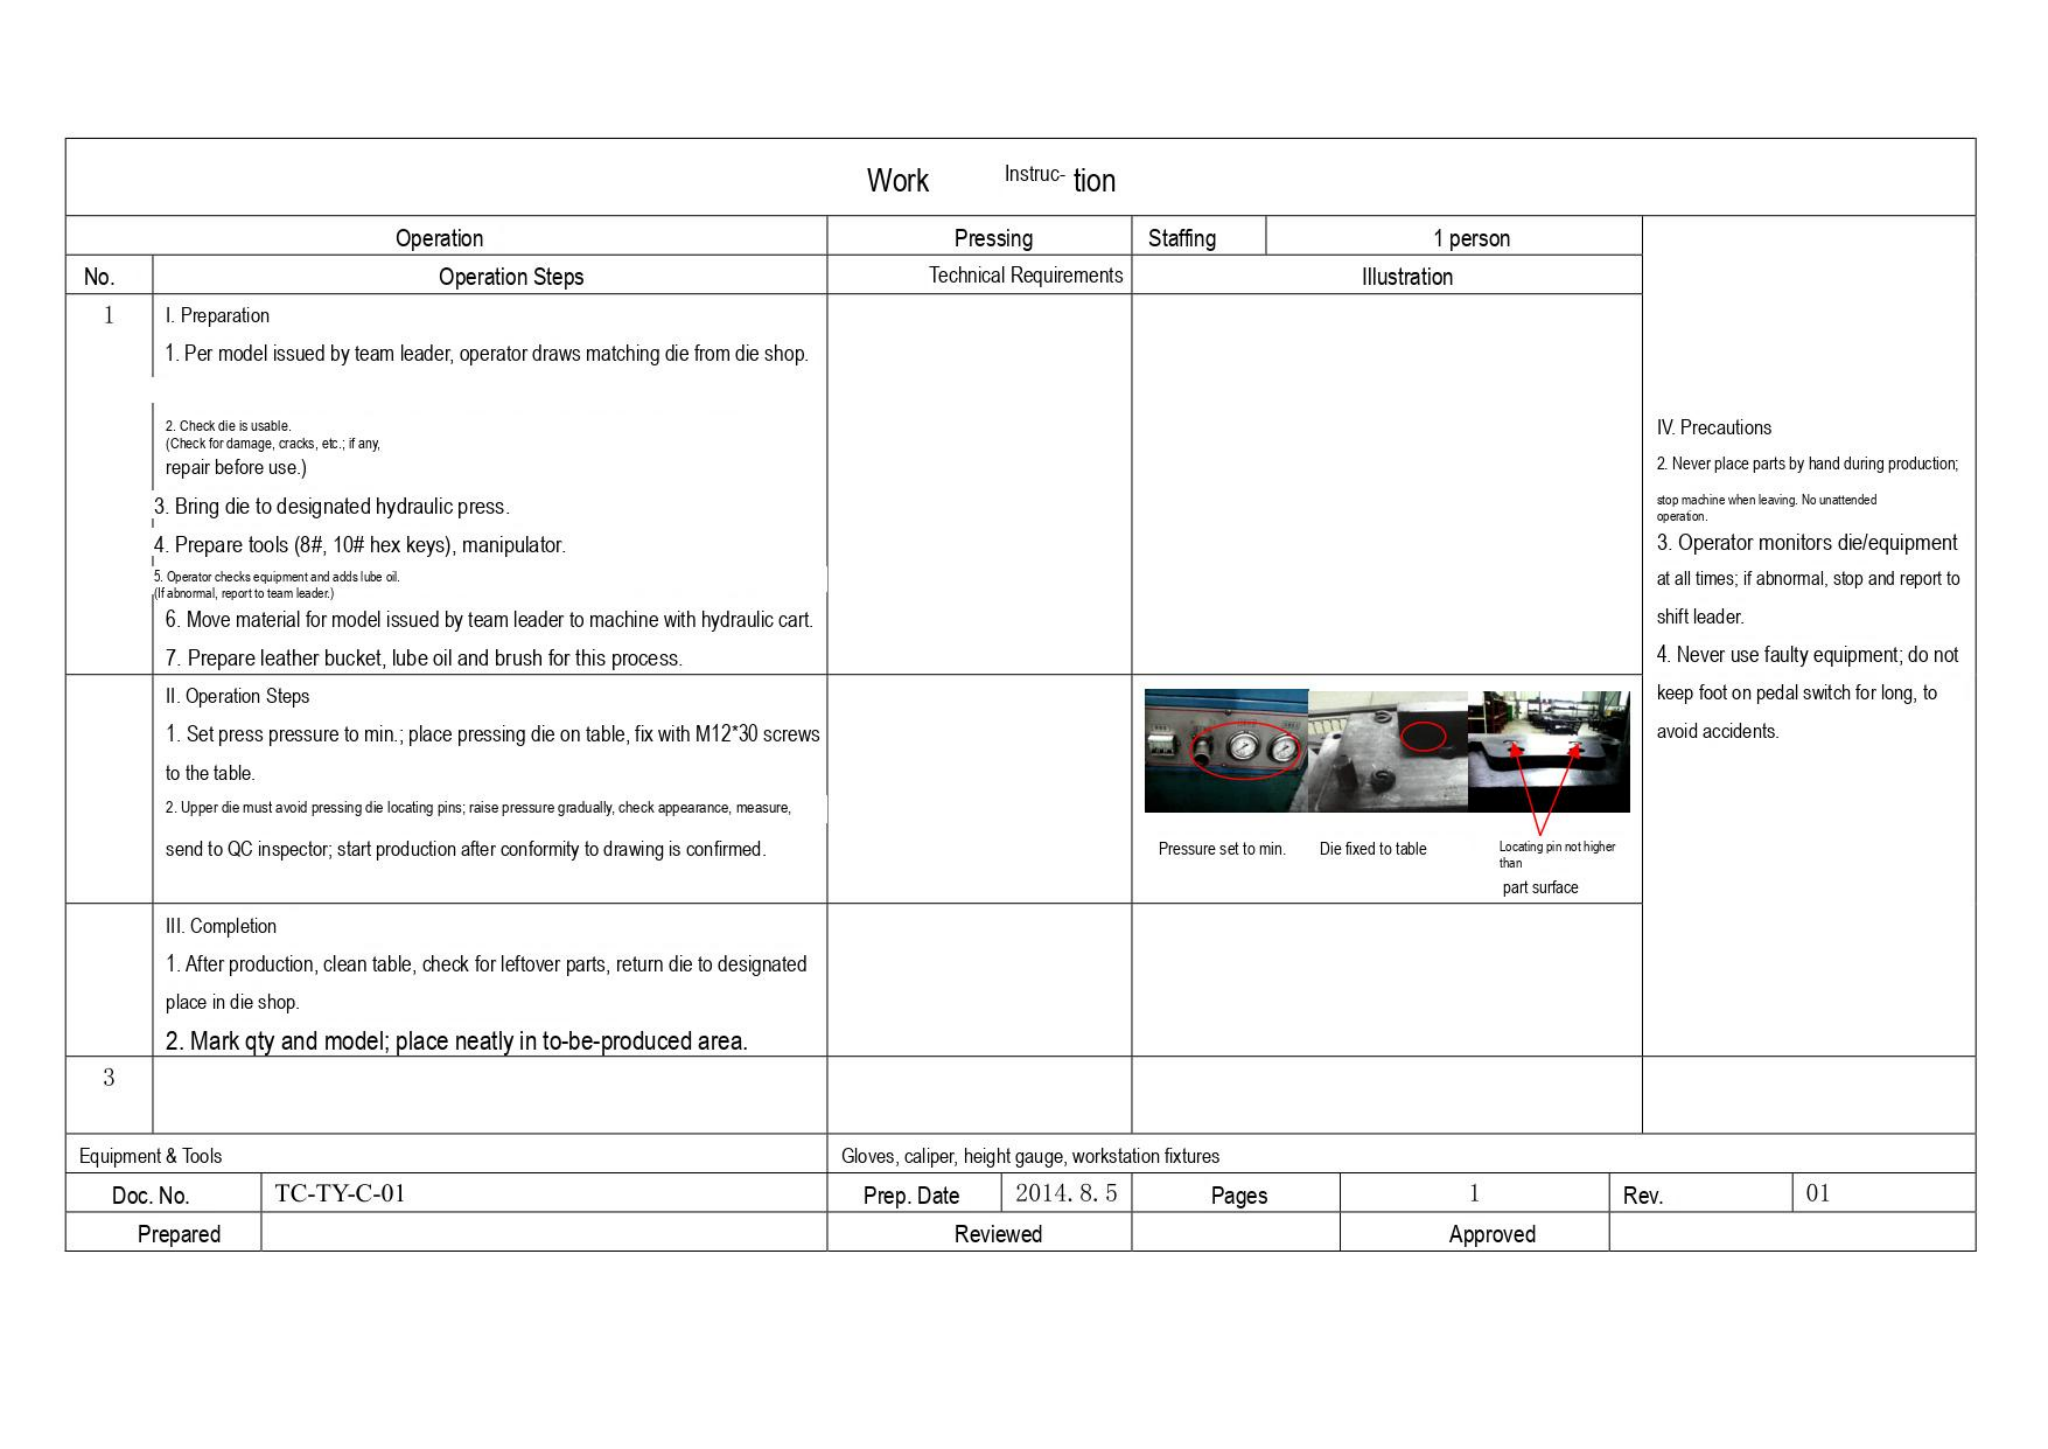Work Instruc- tion

| Operation | | Pressing | Staffing | 1 person | |
|---|---|---|---|---|---|
| No. | Operation Steps | Technical Requirements | Illustration | | IV. Precautions<br>2. Never place parts by hand during production; stop machine when leaving. No unattended operation.<br>3. Operator monitors die/equipment at all times; if abnormal, stop and report to shift leader.<br>4. Never use faulty equipment; do not keep foot on pedal switch for long, to avoid accidents. |
| 1 | I. Preparation<br>1. Per model issued by team leader, operator draws matching die from die shop.<br>2. Check die is usable. (Check for damage, cracks, etc.; if any, repair before use.)<br>3. Bring die to designated hydraulic press.<br>4. Prepare tools (8#, 10# hex keys), manipulator.<br>5. Operator checks equipment and adds lube oil. (If abnormal, report to team leader.)<br>6. Move material for model issued by team leader to machine with hydraulic cart.<br>7. Prepare leather bucket, lube oil and brush for this process. | | | | |
| | II. Operation Steps<br>1. Set press pressure to min.; place pressing die on table, fix with M12*30 screws to the table.<br>2. Upper die must avoid pressing die locating pins; raise pressure gradually, check appearance, measure, send to QC inspector; start production after conformity to drawing is confirmed. | | Pressure set to min.<br>Die fixed to table<br>Locating pin not higher than part surface | | |
| | III. Completion<br>1. After production, clean table, check for leftover parts, return die to designated place in die shop.<br>2. Mark qty and model; place neatly in to-be-produced area. | | | | |
| 3 | | | | | |

| Equipment & Tools | | Gloves, caliper, height gauge, workstation fixtures | | | | | |
|---|---|---|---|---|---|---|---|
| Doc. No. | TC-TY-C-01 | Prep. Date | 2014. 8. 5 | Pages | 1 | Rev. | 01 |
| Prepared | | Reviewed | | | Approved | | |